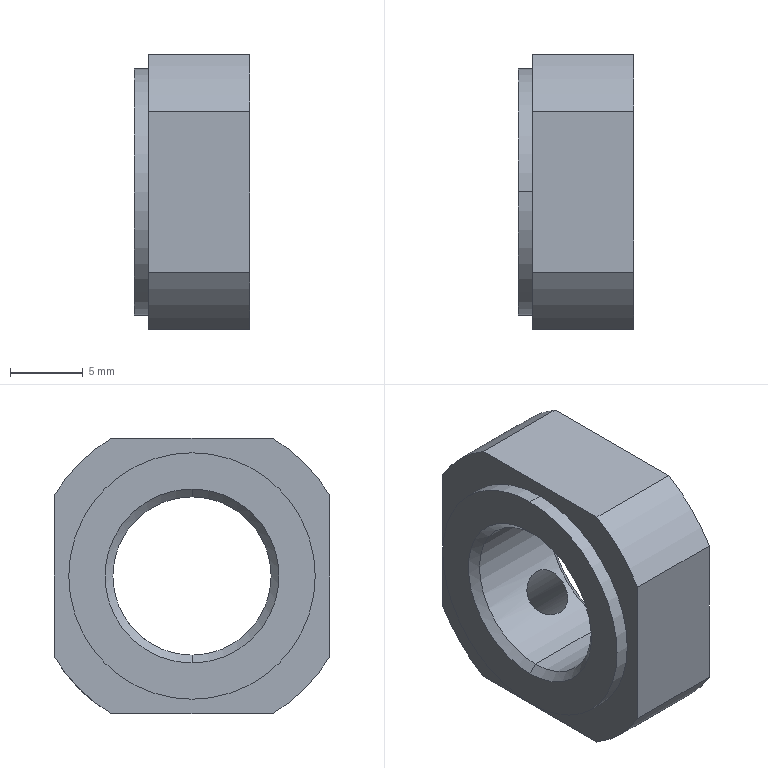Part | SolidWorks | features BaseBody 1 | 1 solid | 23 faces | box 8 x 19 x 19 mm | volume 1767 mm3 | cylinder 10 | plane 7 | cone 6 | commonest cylinder face diameters 22 x4 3.242 x2 10.917 x2 17 x2
STEP:
#1=CARTESIAN_POINT('',(0.,5.545,-9.5));
#2=VERTEX_POINT('',#1);
#3=CARTESIAN_POINT('',(0.,9.5,-5.545));
#4=VERTEX_POINT('',#3);
#5=CARTESIAN_POINT('',(0.,0.,0.));
#6=DIRECTION('',(1.,0.,0.));
#7=DIRECTION('',(0.,0.,-1.));
#8=AXIS2_PLACEMENT_3D('',#5,#6,#7);
#9=CIRCLE('',#8,11.);
#10=EDGE_CURVE('',#2,#4,#9,.T.);
#11=ORIENTED_EDGE('',*,*,#10,.T.);
#12=CARTESIAN_POINT('',(7.,9.5,-5.545));
#13=VERTEX_POINT('',#12);
#14=CARTESIAN_POINT('',(7.,9.5,-5.545));
#15=DIRECTION('',(-1.,0.,0.));
#16=VECTOR('',#15,1000.);
#17=LINE('',#14,#16);
#18=EDGE_CURVE('',#13,#4,#17,.T.);
#19=ORIENTED_EDGE('',*,*,#18,.F.);
#20=CARTESIAN_POINT('',(7.,5.545,-9.5));
#21=VERTEX_POINT('',#20);
#22=CARTESIAN_POINT('',(7.,0.,0.));
#23=DIRECTION('',(1.,0.,0.));
#24=DIRECTION('',(0.,0.,-1.));
#25=AXIS2_PLACEMENT_3D('',#22,#23,#24);
#26=CIRCLE('',#25,11.);
#27=EDGE_CURVE('',#21,#13,#26,.T.);
#28=ORIENTED_EDGE('',*,*,#27,.F.);
#29=CARTESIAN_POINT('',(7.,5.545,-9.5));
#30=DIRECTION('',(-1.,0.,0.));
#31=VECTOR('',#30,1000.);
#32=LINE('',#29,#31);
#33=EDGE_CURVE('',#21,#2,#32,.T.);
#34=ORIENTED_EDGE('',*,*,#33,.T.);
#35=EDGE_LOOP('',(#11,#19,#28,#34));
#36=FACE_OUTER_BOUND('',#35,.T.);
#37=CARTESIAN_POINT('',(4.5,6.364,-8.972));
#38=VERTEX_POINT('',#37);
#39=CARTESIAN_POINT('',(2.966,6.897,-8.569));
#40=VERTEX_POINT('',#39);
#41=CARTESIAN_POINT('',(4.5,6.364,-8.972));
#42=CARTESIAN_POINT('',(4.212,6.364,-8.972));
#43=CARTESIAN_POINT('',(3.926,6.412,-8.939));
#44=CARTESIAN_POINT('',(3.398,6.596,-8.804));
#45=CARTESIAN_POINT('',(3.158,6.732,-8.702));
#46=CARTESIAN_POINT('',(2.966,6.897,-8.569));
#47=B_SPLINE_CURVE_WITH_KNOTS('',3,(#41,#42,#43,#44,#45,#46),.UNSPECIFIED.,.F.,.F.,(4,2,4),(0.8576,0.9288,1.),.UNSPECIFIED.);
#48=EDGE_CURVE('',#38,#40,#47,.T.);
#49=ORIENTED_EDGE('',*,*,#48,.F.);
#50=CARTESIAN_POINT('',(4.5,8.972,-6.364));
#51=VERTEX_POINT('',#50);
#52=CARTESIAN_POINT('',(4.5,8.972,-6.364));
#53=CARTESIAN_POINT('',(4.751,8.972,-6.364));
#54=CARTESIAN_POINT('',(5.004,8.946,-6.401));
#55=CARTESIAN_POINT('',(5.476,8.843,-6.543));
#56=CARTESIAN_POINT('',(5.697,8.765,-6.649));
#57=CARTESIAN_POINT('',(6.073,8.558,-6.913));
#58=CARTESIAN_POINT('',(6.228,8.428,-7.072));
#59=CARTESIAN_POINT('',(6.443,8.127,-7.417));
#60=CARTESIAN_POINT('',(6.5,7.956,-7.601));
#61=CARTESIAN_POINT('',(6.5,7.598,-7.958));
#62=CARTESIAN_POINT('',(6.442,7.414,-8.129));
#63=CARTESIAN_POINT('',(6.228,7.071,-8.429));
#64=CARTESIAN_POINT('',(6.072,6.913,-8.558));
#65=CARTESIAN_POINT('',(5.696,6.649,-8.765));
#66=CARTESIAN_POINT('',(5.476,6.544,-8.843));
#67=CARTESIAN_POINT('',(5.004,6.401,-8.946));
#68=CARTESIAN_POINT('',(4.753,6.364,-8.972));
#69=CARTESIAN_POINT('',(4.5,6.364,-8.972));
#70=B_SPLINE_CURVE_WITH_KNOTS('',3,(#52,#53,#54,#55,#56,#57,#58,#59,#60,#61,#62,#63,#64,#65,#66,#67,#68,#69),.UNSPECIFIED.,.F.,.F.,(4,2,2,2,2,2,2,2,4),(0.3577,0.4202,0.4827,0.5452,0.6076,0.6701,0.7326,0.7951,0.8576),.UNSPECIFIED.);
#71=EDGE_CURVE('',#51,#38,#70,.T.);
#72=ORIENTED_EDGE('',*,*,#71,.F.);
#73=CARTESIAN_POINT('',(2.966,6.897,-8.569));
#74=CARTESIAN_POINT('',(2.846,7.001,-8.485));
#75=CARTESIAN_POINT('',(2.744,7.118,-8.388));
#76=CARTESIAN_POINT('',(2.59,7.363,-8.174));
#77=CARTESIAN_POINT('',(2.538,7.493,-8.055));
#78=CARTESIAN_POINT('',(2.491,7.751,-7.808));
#79=CARTESIAN_POINT('',(2.497,7.879,-7.678));
#80=CARTESIAN_POINT('',(2.564,8.122,-7.42));
#81=CARTESIAN_POINT('',(2.626,8.237,-7.293));
#82=CARTESIAN_POINT('',(2.885,8.547,-6.932));
#83=CARTESIAN_POINT('',(3.151,8.707,-6.725));
#84=CARTESIAN_POINT('',(3.78,8.919,-6.44));
#85=CARTESIAN_POINT('',(4.14,8.972,-6.364));
#86=CARTESIAN_POINT('',(4.5,8.972,-6.364));
#87=B_SPLINE_CURVE_WITH_KNOTS('',3,(#73,#74,#75,#76,#77,#78,#79,#80,#81,#82,#83,#84,#85,#86),.UNSPECIFIED.,.F.,.F.,(4,2,2,2,2,2,4),(0.,0.04471,0.08942,0.1341,0.1788,0.2683,0.3577),.UNSPECIFIED.);
#88=EDGE_CURVE('',#40,#51,#87,.T.);
#89=ORIENTED_EDGE('',*,*,#88,.F.);
#90=EDGE_LOOP('',(#49,#72,#89));
#91=FACE_BOUND('',#90,.T.);
#92=CARTESIAN_POINT('',(7.,0.,0.));
#93=DIRECTION('',(-1.,0.,0.));
#94=DIRECTION('',(0.,-0.7071,0.7071));
#95=AXIS2_PLACEMENT_3D('',#92,#93,#94);
#96=CYLINDRICAL_SURFACE('',#95,11.);
#97=ADVANCED_FACE('',(#36,#91),#96,.T.);
#98=CARTESIAN_POINT('',(4.5,6.364,-8.656));
#99=VERTEX_POINT('',#98);
#100=CARTESIAN_POINT('',(4.5,6.364,-8.656));
#101=DIRECTION('',(0.,0.,-1.));
#102=VECTOR('',#101,1000.);
#103=LINE('',#100,#102);
#104=EDGE_CURVE('',#99,#38,#103,.T.);
#105=ORIENTED_EDGE('',*,*,#104,.T.);
#106=ORIENTED_EDGE('',*,*,#48,.T.);
#107=ORIENTED_EDGE('',*,*,#88,.T.);
#108=CARTESIAN_POINT('',(4.5,8.656,-6.364));
#109=VERTEX_POINT('',#108);
#110=CARTESIAN_POINT('',(4.5,8.656,-6.364));
#111=DIRECTION('',(0.,1.,0.));
#112=VECTOR('',#111,1000.);
#113=LINE('',#110,#112);
#114=EDGE_CURVE('',#109,#51,#113,.T.);
#115=ORIENTED_EDGE('',*,*,#114,.F.);
#116=CARTESIAN_POINT('',(4.5,7.51,-7.51));
#117=DIRECTION('',(0.,-0.7071,0.7071));
#118=DIRECTION('',(0.,-0.7071,-0.7071));
#119=AXIS2_PLACEMENT_3D('',#116,#117,#118);
#120=CIRCLE('',#119,1.621);
#121=EDGE_CURVE('',#109,#99,#120,.T.);
#122=ORIENTED_EDGE('',*,*,#121,.T.);
#123=EDGE_LOOP('',(#105,#106,#107,#115,#122));
#124=FACE_OUTER_BOUND('',#123,.T.);
#125=CARTESIAN_POINT('',(4.5,7.778,-7.778));
#126=DIRECTION('',(0.,0.7071,-0.7071));
#127=DIRECTION('',(1.,0.,0.));
#128=AXIS2_PLACEMENT_3D('',#125,#126,#127);
#129=CONICAL_SURFACE('',#128,2.,0.7854);
#130=ADVANCED_FACE('',(#124),#129,.F.);
#131=CARTESIAN_POINT('',(4.5,4.832,-2.539));
#132=VERTEX_POINT('',#131);
#133=CARTESIAN_POINT('',(4.5,8.656,-6.364));
#134=DIRECTION('',(0.,-0.7071,0.7071));
#135=VECTOR('',#134,1000.);
#136=LINE('',#133,#135);
#137=EDGE_CURVE('',#109,#132,#136,.T.);
#138=ORIENTED_EDGE('',*,*,#137,.T.);
#139=CARTESIAN_POINT('',(4.5,2.539,-4.832));
#140=VERTEX_POINT('',#139);
#141=CARTESIAN_POINT('',(4.5,2.539,-4.832));
#142=CARTESIAN_POINT('',(4.288,2.539,-4.832));
#143=CARTESIAN_POINT('',(4.074,2.579,-4.811));
#144=CARTESIAN_POINT('',(3.682,2.728,-4.729));
#145=CARTESIAN_POINT('',(3.504,2.835,-4.667));
#146=CARTESIAN_POINT('',(3.205,3.091,-4.501));
#147=CARTESIAN_POINT('',(3.085,3.24,-4.398));
#148=CARTESIAN_POINT('',(2.922,3.549,-4.152));
#149=CARTESIAN_POINT('',(2.879,3.709,-4.011));
#150=CARTESIAN_POINT('',(2.879,4.011,-3.708));
#151=CARTESIAN_POINT('',(2.922,4.153,-3.548));
#152=CARTESIAN_POINT('',(3.085,4.397,-3.24));
#153=CARTESIAN_POINT('',(3.205,4.501,-3.091));
#154=CARTESIAN_POINT('',(3.503,4.667,-2.835));
#155=CARTESIAN_POINT('',(3.681,4.729,-2.728));
#156=CARTESIAN_POINT('',(4.074,4.811,-2.58));
#157=CARTESIAN_POINT('',(4.286,4.832,-2.54));
#158=CARTESIAN_POINT('',(4.5,4.832,-2.539));
#159=B_SPLINE_CURVE_WITH_KNOTS('',3,(#141,#142,#143,#144,#145,#146,#147,#148,#149,#150,#151,#152,#153,#154,#155,#156,#157,#158),.UNSPECIFIED.,.F.,.F.,(4,2,2,2,2,2,2,2,4),(0.,0.0625,0.125,0.1875,0.25,0.3125,0.375,0.4375,0.5),.UNSPECIFIED.);
#160=EDGE_CURVE('',#140,#132,#159,.T.);
#161=ORIENTED_EDGE('',*,*,#160,.F.);
#162=CARTESIAN_POINT('',(4.5,6.364,-8.656));
#163=DIRECTION('',(0.,-0.7071,0.7071));
#164=VECTOR('',#163,1000.);
#165=LINE('',#162,#164);
#166=EDGE_CURVE('',#99,#140,#165,.T.);
#167=ORIENTED_EDGE('',*,*,#166,.F.);
#168=ORIENTED_EDGE('',*,*,#121,.F.);
#169=EDGE_LOOP('',(#138,#161,#167,#168));
#170=FACE_OUTER_BOUND('',#169,.T.);
#171=CARTESIAN_POINT('',(4.5,0.,0.));
#172=DIRECTION('',(0.,-0.7071,0.7071));
#173=DIRECTION('',(1.,0.,0.));
#174=AXIS2_PLACEMENT_3D('',#171,#172,#173);
#175=CYLINDRICAL_SURFACE('',#174,1.621);
#176=ADVANCED_FACE('',(#170),#175,.F.);
#177=ORIENTED_EDGE('',*,*,#137,.F.);
#178=CARTESIAN_POINT('',(4.5,7.51,-7.51));
#179=DIRECTION('',(0.,-0.7071,0.7071));
#180=DIRECTION('',(0.,-0.7071,-0.7071));
#181=AXIS2_PLACEMENT_3D('',#178,#179,#180);
#182=CIRCLE('',#181,1.621);
#183=EDGE_CURVE('',#99,#109,#182,.T.);
#184=ORIENTED_EDGE('',*,*,#183,.F.);
#185=ORIENTED_EDGE('',*,*,#166,.T.);
#186=CARTESIAN_POINT('',(4.5,4.832,-2.539));
#187=CARTESIAN_POINT('',(4.714,4.832,-2.54));
#188=CARTESIAN_POINT('',(4.926,4.811,-2.58));
#189=CARTESIAN_POINT('',(5.319,4.729,-2.728));
#190=CARTESIAN_POINT('',(5.497,4.667,-2.835));
#191=CARTESIAN_POINT('',(5.795,4.502,-3.091));
#192=CARTESIAN_POINT('',(5.916,4.397,-3.241));
#193=CARTESIAN_POINT('',(6.078,4.153,-3.548));
#194=CARTESIAN_POINT('',(6.121,4.011,-3.709));
#195=CARTESIAN_POINT('',(6.121,3.709,-4.011));
#196=CARTESIAN_POINT('',(6.078,3.549,-4.152));
#197=CARTESIAN_POINT('',(5.915,3.24,-4.398));
#198=CARTESIAN_POINT('',(5.795,3.091,-4.501));
#199=CARTESIAN_POINT('',(5.496,2.835,-4.667));
#200=CARTESIAN_POINT('',(5.318,2.728,-4.729));
#201=CARTESIAN_POINT('',(4.926,2.579,-4.811));
#202=CARTESIAN_POINT('',(4.712,2.539,-4.832));
#203=CARTESIAN_POINT('',(4.5,2.539,-4.832));
#204=B_SPLINE_CURVE_WITH_KNOTS('',3,(#186,#187,#188,#189,#190,#191,#192,#193,#194,#195,#196,#197,#198,#199,#200,#201,#202,#203),.UNSPECIFIED.,.F.,.F.,(4,2,2,2,2,2,2,2,4),(0.5,0.5625,0.625,0.6875,0.75,0.8125,0.875,0.9375,1.),.UNSPECIFIED.);
#205=EDGE_CURVE('',#132,#140,#204,.T.);
#206=ORIENTED_EDGE('',*,*,#205,.F.);
#207=EDGE_LOOP('',(#177,#184,#185,#206));
#208=FACE_OUTER_BOUND('',#207,.T.);
#209=CARTESIAN_POINT('',(4.5,0.,0.));
#210=DIRECTION('',(0.,-0.7071,0.7071));
#211=DIRECTION('',(-1.,0.,0.));
#212=AXIS2_PLACEMENT_3D('',#209,#210,#211);
#213=CYLINDRICAL_SURFACE('',#212,1.621);
#214=ADVANCED_FACE('',(#208),#213,.F.);
#215=CARTESIAN_POINT('',(-0.4585,0.,5.458));
#216=VERTEX_POINT('',#215);
#217=CARTESIAN_POINT('',(6.459,0.,5.458));
#218=VERTEX_POINT('',#217);
#219=CARTESIAN_POINT('',(-0.4585,0.,5.458));
#220=DIRECTION('',(1.,0.,0.));
#221=VECTOR('',#220,1000.);
#222=LINE('',#219,#221);
#223=EDGE_CURVE('',#216,#218,#222,.T.);
#224=ORIENTED_EDGE('',*,*,#223,.F.);
#225=CARTESIAN_POINT('',(-0.4585,0.,-5.458));
#226=VERTEX_POINT('',#225);
#227=CARTESIAN_POINT('',(-0.4585,0.,0.));
#228=DIRECTION('',(1.,0.,0.));
#229=DIRECTION('',(0.,0.,-1.));
#230=AXIS2_PLACEMENT_3D('',#227,#228,#229);
#231=CIRCLE('',#230,5.458);
#232=EDGE_CURVE('',#226,#216,#231,.T.);
#233=ORIENTED_EDGE('',*,*,#232,.F.);
#234=CARTESIAN_POINT('',(6.458,0.,-5.458));
#235=VERTEX_POINT('',#234);
#236=CARTESIAN_POINT('',(-0.4585,0.,-5.458));
#237=DIRECTION('',(1.,0.,0.));
#238=VECTOR('',#237,1000.);
#239=LINE('',#236,#238);
#240=EDGE_CURVE('',#226,#235,#239,.T.);
#241=ORIENTED_EDGE('',*,*,#240,.T.);
#242=CARTESIAN_POINT('',(6.458,0.,0.));
#243=DIRECTION('',(1.,0.,0.));
#244=DIRECTION('',(0.,0.,-1.));
#245=AXIS2_PLACEMENT_3D('',#242,#243,#244);
#246=CIRCLE('',#245,5.458);
#247=EDGE_CURVE('',#235,#218,#246,.T.);
#248=ORIENTED_EDGE('',*,*,#247,.T.);
#249=EDGE_LOOP('',(#224,#233,#241,#248));
#250=FACE_OUTER_BOUND('',#249,.T.);
#251=ORIENTED_EDGE('',*,*,#160,.T.);
#252=ORIENTED_EDGE('',*,*,#205,.T.);
#253=EDGE_LOOP('',(#251,#252));
#254=FACE_BOUND('',#253,.T.);
#255=CARTESIAN_POINT('',(7.,0.,0.));
#256=DIRECTION('',(1.,0.,0.));
#257=DIRECTION('',(0.,-1.,0.));
#258=AXIS2_PLACEMENT_3D('',#255,#256,#257);
#259=CYLINDRICAL_SURFACE('',#258,5.458);
#260=ADVANCED_FACE('',(#250,#254),#259,.F.);
#261=CARTESIAN_POINT('',(7.,0.,6.));
#262=VERTEX_POINT('',#261);
#263=CARTESIAN_POINT('',(6.458,0.,5.458));
#264=DIRECTION('',(0.7071,0.,0.7071));
#265=VECTOR('',#264,1000.);
#266=LINE('',#263,#265);
#267=EDGE_CURVE('',#218,#262,#266,.T.);
#268=ORIENTED_EDGE('',*,*,#267,.F.);
#269=ORIENTED_EDGE('',*,*,#247,.F.);
#270=CARTESIAN_POINT('',(7.,0.,-6.));
#271=VERTEX_POINT('',#270);
#272=CARTESIAN_POINT('',(6.458,0.,-5.458));
#273=DIRECTION('',(0.7071,0.,-0.7071));
#274=VECTOR('',#273,1000.);
#275=LINE('',#272,#274);
#276=EDGE_CURVE('',#235,#271,#275,.T.);
#277=ORIENTED_EDGE('',*,*,#276,.T.);
#278=CARTESIAN_POINT('',(7.,0.,0.));
#279=DIRECTION('',(1.,0.,0.));
#280=DIRECTION('',(0.,0.,-1.));
#281=AXIS2_PLACEMENT_3D('',#278,#279,#280);
#282=CIRCLE('',#281,6.);
#283=EDGE_CURVE('',#271,#262,#282,.T.);
#284=ORIENTED_EDGE('',*,*,#283,.T.);
#285=EDGE_LOOP('',(#268,#269,#277,#284));
#286=FACE_OUTER_BOUND('',#285,.T.);
#287=CARTESIAN_POINT('',(6.458,0.,0.));
#288=DIRECTION('',(1.,0.,0.));
#289=DIRECTION('',(0.,-1.,0.));
#290=AXIS2_PLACEMENT_3D('',#287,#288,#289);
#291=CONICAL_SURFACE('',#290,5.458,0.7854);
#292=ADVANCED_FACE('',(#286),#291,.F.);
#293=CARTESIAN_POINT('',(7.,0.,0.));
#294=DIRECTION('',(1.,0.,0.));
#295=DIRECTION('',(0.,0.,-1.));
#296=AXIS2_PLACEMENT_3D('',#293,#294,#295);
#297=CIRCLE('',#296,6.);
#298=EDGE_CURVE('',#262,#271,#297,.T.);
#299=ORIENTED_EDGE('',*,*,#298,.F.);
#300=ORIENTED_EDGE('',*,*,#283,.F.);
#301=EDGE_LOOP('',(#299,#300));
#302=FACE_BOUND('',#301,.T.);
#303=CARTESIAN_POINT('',(7.,9.5,5.545));
#304=VERTEX_POINT('',#303);
#305=CARTESIAN_POINT('',(7.,5.545,9.5));
#306=VERTEX_POINT('',#305);
#307=CARTESIAN_POINT('',(7.,0.,0.));
#308=DIRECTION('',(1.,0.,0.));
#309=DIRECTION('',(0.,0.,-1.));
#310=AXIS2_PLACEMENT_3D('',#307,#308,#309);
#311=CIRCLE('',#310,11.);
#312=EDGE_CURVE('',#304,#306,#311,.T.);
#313=ORIENTED_EDGE('',*,*,#312,.T.);
#314=CARTESIAN_POINT('',(7.,-5.545,9.5));
#315=VERTEX_POINT('',#314);
#316=CARTESIAN_POINT('',(7.,5.545,9.5));
#317=DIRECTION('',(0.,-1.,0.));
#318=VECTOR('',#317,1000.);
#319=LINE('',#316,#318);
#320=EDGE_CURVE('',#306,#315,#319,.T.);
#321=ORIENTED_EDGE('',*,*,#320,.T.);
#322=CARTESIAN_POINT('',(7.,-9.5,5.545));
#323=VERTEX_POINT('',#322);
#324=CARTESIAN_POINT('',(7.,0.,0.));
#325=DIRECTION('',(1.,0.,0.));
#326=DIRECTION('',(0.,0.,-1.));
#327=AXIS2_PLACEMENT_3D('',#324,#325,#326);
#328=CIRCLE('',#327,11.);
#329=EDGE_CURVE('',#315,#323,#328,.T.);
#330=ORIENTED_EDGE('',*,*,#329,.T.);
#331=CARTESIAN_POINT('',(7.,-9.5,-5.545));
#332=VERTEX_POINT('',#331);
#333=CARTESIAN_POINT('',(7.,-9.5,5.545));
#334=DIRECTION('',(0.,0.,-1.));
#335=VECTOR('',#334,1000.);
#336=LINE('',#333,#335);
#337=EDGE_CURVE('',#323,#332,#336,.T.);
#338=ORIENTED_EDGE('',*,*,#337,.T.);
#339=CARTESIAN_POINT('',(7.,-5.545,-9.5));
#340=VERTEX_POINT('',#339);
#341=CARTESIAN_POINT('',(7.,0.,0.));
#342=DIRECTION('',(1.,0.,0.));
#343=DIRECTION('',(0.,0.,-1.));
#344=AXIS2_PLACEMENT_3D('',#341,#342,#343);
#345=CIRCLE('',#344,11.);
#346=EDGE_CURVE('',#332,#340,#345,.T.);
#347=ORIENTED_EDGE('',*,*,#346,.T.);
#348=CARTESIAN_POINT('',(7.,-5.545,-9.5));
#349=DIRECTION('',(0.,1.,0.));
#350=VECTOR('',#349,1000.);
#351=LINE('',#348,#350);
#352=EDGE_CURVE('',#340,#21,#351,.T.);
#353=ORIENTED_EDGE('',*,*,#352,.T.);
#354=ORIENTED_EDGE('',*,*,#27,.T.);
#355=CARTESIAN_POINT('',(7.,9.5,-5.545));
#356=DIRECTION('',(0.,0.,1.));
#357=VECTOR('',#356,1000.);
#358=LINE('',#355,#357);
#359=EDGE_CURVE('',#13,#304,#358,.T.);
#360=ORIENTED_EDGE('',*,*,#359,.T.);
#361=EDGE_LOOP('',(#313,#321,#330,#338,#347,#353,#354,#360));
#362=FACE_OUTER_BOUND('',#361,.T.);
#363=CARTESIAN_POINT('',(7.,0.,0.));
#364=DIRECTION('',(1.,0.,0.));
#365=DIRECTION('',(0.,0.,-1.));
#366=AXIS2_PLACEMENT_3D('',#363,#364,#365);
#367=PLANE('',#366);
#368=ADVANCED_FACE('',(#302,#362),#367,.T.);
#369=CARTESIAN_POINT('',(0.,9.5,5.545));
#370=VERTEX_POINT('',#369);
#371=CARTESIAN_POINT('',(0.,9.5,-5.545));
#372=DIRECTION('',(0.,0.,1.));
#373=VECTOR('',#372,1000.);
#374=LINE('',#371,#373);
#375=EDGE_CURVE('',#4,#370,#374,.T.);
#376=ORIENTED_EDGE('',*,*,#375,.T.);
#377=CARTESIAN_POINT('',(7.,9.5,5.545));
#378=DIRECTION('',(-1.,0.,0.));
#379=VECTOR('',#378,1000.);
#380=LINE('',#377,#379);
#381=EDGE_CURVE('',#304,#370,#380,.T.);
#382=ORIENTED_EDGE('',*,*,#381,.F.);
#383=ORIENTED_EDGE('',*,*,#359,.F.);
#384=ORIENTED_EDGE('',*,*,#18,.T.);
#385=EDGE_LOOP('',(#376,#382,#383,#384));
#386=FACE_OUTER_BOUND('',#385,.T.);
#387=CARTESIAN_POINT('',(7.,9.5,-5.545));
#388=DIRECTION('',(0.,-1.,0.));
#389=DIRECTION('',(0.,0.,-1.));
#390=AXIS2_PLACEMENT_3D('',#387,#388,#389);
#391=PLANE('',#390);
#392=ADVANCED_FACE('',(#386),#391,.F.);
#393=CARTESIAN_POINT('',(0.,5.545,9.5));
#394=VERTEX_POINT('',#393);
#395=CARTESIAN_POINT('',(0.,0.,0.));
#396=DIRECTION('',(1.,0.,0.));
#397=DIRECTION('',(0.,0.,-1.));
#398=AXIS2_PLACEMENT_3D('',#395,#396,#397);
#399=CIRCLE('',#398,11.);
#400=EDGE_CURVE('',#370,#394,#399,.T.);
#401=ORIENTED_EDGE('',*,*,#400,.T.);
#402=CARTESIAN_POINT('',(7.,5.545,9.5));
#403=DIRECTION('',(-1.,0.,0.));
#404=VECTOR('',#403,1000.);
#405=LINE('',#402,#404);
#406=EDGE_CURVE('',#306,#394,#405,.T.);
#407=ORIENTED_EDGE('',*,*,#406,.F.);
#408=ORIENTED_EDGE('',*,*,#312,.F.);
#409=ORIENTED_EDGE('',*,*,#381,.T.);
#410=EDGE_LOOP('',(#401,#407,#408,#409));
#411=FACE_OUTER_BOUND('',#410,.T.);
#412=CARTESIAN_POINT('',(7.,0.,0.));
#413=DIRECTION('',(-1.,0.,0.));
#414=DIRECTION('',(0.,-0.7071,-0.7071));
#415=AXIS2_PLACEMENT_3D('',#412,#413,#414);
#416=CYLINDRICAL_SURFACE('',#415,11.);
#417=ADVANCED_FACE('',(#411),#416,.T.);
#418=CARTESIAN_POINT('',(0.,-5.545,9.5));
#419=VERTEX_POINT('',#418);
#420=CARTESIAN_POINT('',(0.,5.545,9.5));
#421=DIRECTION('',(0.,-1.,0.));
#422=VECTOR('',#421,1000.);
#423=LINE('',#420,#422);
#424=EDGE_CURVE('',#394,#419,#423,.T.);
#425=ORIENTED_EDGE('',*,*,#424,.T.);
#426=CARTESIAN_POINT('',(7.,-5.545,9.5));
#427=DIRECTION('',(-1.,0.,0.));
#428=VECTOR('',#427,1000.);
#429=LINE('',#426,#428);
#430=EDGE_CURVE('',#315,#419,#429,.T.);
#431=ORIENTED_EDGE('',*,*,#430,.F.);
#432=ORIENTED_EDGE('',*,*,#320,.F.);
#433=ORIENTED_EDGE('',*,*,#406,.T.);
#434=EDGE_LOOP('',(#425,#431,#432,#433));
#435=FACE_OUTER_BOUND('',#434,.T.);
#436=CARTESIAN_POINT('',(7.,5.545,9.5));
#437=DIRECTION('',(0.,0.,-1.));
#438=DIRECTION('',(-1.,0.,0.));
#439=AXIS2_PLACEMENT_3D('',#436,#437,#438);
#440=PLANE('',#439);
#441=ADVANCED_FACE('',(#435),#440,.F.);
#442=CARTESIAN_POINT('',(0.,-9.5,5.545));
#443=VERTEX_POINT('',#442);
#444=CARTESIAN_POINT('',(0.,0.,0.));
#445=DIRECTION('',(1.,0.,0.));
#446=DIRECTION('',(0.,0.,-1.));
#447=AXIS2_PLACEMENT_3D('',#444,#445,#446);
#448=CIRCLE('',#447,11.);
#449=EDGE_CURVE('',#419,#443,#448,.T.);
#450=ORIENTED_EDGE('',*,*,#449,.T.);
#451=CARTESIAN_POINT('',(7.,-9.5,5.545));
#452=DIRECTION('',(-1.,0.,0.));
#453=VECTOR('',#452,1000.);
#454=LINE('',#451,#453);
#455=EDGE_CURVE('',#323,#443,#454,.T.);
#456=ORIENTED_EDGE('',*,*,#455,.F.);
#457=ORIENTED_EDGE('',*,*,#329,.F.);
#458=ORIENTED_EDGE('',*,*,#430,.T.);
#459=EDGE_LOOP('',(#450,#456,#457,#458));
#460=FACE_OUTER_BOUND('',#459,.T.);
#461=CARTESIAN_POINT('',(7.,0.,0.));
#462=DIRECTION('',(-1.,0.,0.));
#463=DIRECTION('',(0.,0.7071,-0.7071));
#464=AXIS2_PLACEMENT_3D('',#461,#462,#463);
#465=CYLINDRICAL_SURFACE('',#464,11.);
#466=ADVANCED_FACE('',(#460),#465,.T.);
#467=CARTESIAN_POINT('',(0.,-9.5,-5.545));
#468=VERTEX_POINT('',#467);
#469=CARTESIAN_POINT('',(0.,-9.5,5.545));
#470=DIRECTION('',(0.,0.,-1.));
#471=VECTOR('',#470,1000.);
#472=LINE('',#469,#471);
#473=EDGE_CURVE('',#443,#468,#472,.T.);
#474=ORIENTED_EDGE('',*,*,#473,.T.);
#475=CARTESIAN_POINT('',(7.,-9.5,-5.545));
#476=DIRECTION('',(-1.,0.,0.));
#477=VECTOR('',#476,1000.);
#478=LINE('',#475,#477);
#479=EDGE_CURVE('',#332,#468,#478,.T.);
#480=ORIENTED_EDGE('',*,*,#479,.F.);
#481=ORIENTED_EDGE('',*,*,#337,.F.);
#482=ORIENTED_EDGE('',*,*,#455,.T.);
#483=EDGE_LOOP('',(#474,#480,#481,#482));
#484=FACE_OUTER_BOUND('',#483,.T.);
#485=CARTESIAN_POINT('',(7.,-9.5,5.545));
#486=DIRECTION('',(0.,1.,0.));
#487=DIRECTION('',(0.,0.,1.));
#488=AXIS2_PLACEMENT_3D('',#485,#486,#487);
#489=PLANE('',#488);
#490=ADVANCED_FACE('',(#484),#489,.F.);
#491=CARTESIAN_POINT('',(0.,-5.545,-9.5));
#492=VERTEX_POINT('',#491);
#493=CARTESIAN_POINT('',(0.,0.,0.));
#494=DIRECTION('',(1.,0.,0.));
#495=DIRECTION('',(0.,0.,-1.));
#496=AXIS2_PLACEMENT_3D('',#493,#494,#495);
#497=CIRCLE('',#496,11.);
#498=EDGE_CURVE('',#468,#492,#497,.T.);
#499=ORIENTED_EDGE('',*,*,#498,.T.);
#500=CARTESIAN_POINT('',(7.,-5.545,-9.5));
#501=DIRECTION('',(-1.,0.,0.));
#502=VECTOR('',#501,1000.);
#503=LINE('',#500,#502);
#504=EDGE_CURVE('',#340,#492,#503,.T.);
#505=ORIENTED_EDGE('',*,*,#504,.F.);
#506=ORIENTED_EDGE('',*,*,#346,.F.);
#507=ORIENTED_EDGE('',*,*,#479,.T.);
#508=EDGE_LOOP('',(#499,#505,#506,#507));
#509=FACE_OUTER_BOUND('',#508,.T.);
#510=CARTESIAN_POINT('',(7.,0.,0.));
#511=DIRECTION('',(-1.,0.,0.));
#512=DIRECTION('',(0.,0.7071,0.7071));
#513=AXIS2_PLACEMENT_3D('',#510,#511,#512);
#514=CYLINDRICAL_SURFACE('',#513,11.);
#515=ADVANCED_FACE('',(#509),#514,.T.);
#516=CARTESIAN_POINT('',(0.,-5.545,-9.5));
#517=DIRECTION('',(0.,1.,0.));
#518=VECTOR('',#517,1000.);
#519=LINE('',#516,#518);
#520=EDGE_CURVE('',#492,#2,#519,.T.);
#521=ORIENTED_EDGE('',*,*,#520,.T.);
#522=ORIENTED_EDGE('',*,*,#33,.F.);
#523=ORIENTED_EDGE('',*,*,#352,.F.);
#524=ORIENTED_EDGE('',*,*,#504,.T.);
#525=EDGE_LOOP('',(#521,#522,#523,#524));
#526=FACE_OUTER_BOUND('',#525,.T.);
#527=CARTESIAN_POINT('',(7.,-5.545,-9.5));
#528=DIRECTION('',(0.,0.,1.));
#529=DIRECTION('',(1.,0.,0.));
#530=AXIS2_PLACEMENT_3D('',#527,#528,#529);
#531=PLANE('',#530);
#532=ADVANCED_FACE('',(#526),#531,.F.);
#533=CARTESIAN_POINT('',(0.,0.,8.5));
#534=VERTEX_POINT('',#533);
#535=CARTESIAN_POINT('',(0.,0.,-8.5));
#536=VERTEX_POINT('',#535);
#537=CARTESIAN_POINT('',(0.,0.,0.));
#538=DIRECTION('',(-1.,0.,0.));
#539=DIRECTION('',(0.,0.,-1.));
#540=AXIS2_PLACEMENT_3D('',#537,#538,#539);
#541=CIRCLE('',#540,8.5);
#542=EDGE_CURVE('',#534,#536,#541,.T.);
#543=ORIENTED_EDGE('',*,*,#542,.F.);
#544=CARTESIAN_POINT('',(0.,0.,0.));
#545=DIRECTION('',(-1.,0.,0.));
#546=DIRECTION('',(0.,0.,-1.));
#547=AXIS2_PLACEMENT_3D('',#544,#545,#546);
#548=CIRCLE('',#547,8.5);
#549=EDGE_CURVE('',#536,#534,#548,.T.);
#550=ORIENTED_EDGE('',*,*,#549,.F.);
#551=EDGE_LOOP('',(#543,#550));
#552=FACE_BOUND('',#551,.T.);
#553=ORIENTED_EDGE('',*,*,#400,.F.);
#554=ORIENTED_EDGE('',*,*,#375,.F.);
#555=ORIENTED_EDGE('',*,*,#10,.F.);
#556=ORIENTED_EDGE('',*,*,#520,.F.);
#557=ORIENTED_EDGE('',*,*,#498,.F.);
#558=ORIENTED_EDGE('',*,*,#473,.F.);
#559=ORIENTED_EDGE('',*,*,#449,.F.);
#560=ORIENTED_EDGE('',*,*,#424,.F.);
#561=EDGE_LOOP('',(#553,#554,#555,#556,#557,#558,#559,#560));
#562=FACE_OUTER_BOUND('',#561,.T.);
#563=CARTESIAN_POINT('',(0.,0.,0.));
#564=DIRECTION('',(1.,0.,0.));
#565=DIRECTION('',(0.,0.,-1.));
#566=AXIS2_PLACEMENT_3D('',#563,#564,#565);
#567=PLANE('',#566);
#568=ADVANCED_FACE('',(#552,#562),#567,.F.);
#569=CARTESIAN_POINT('',(-1.,0.,8.5));
#570=VERTEX_POINT('',#569);
#571=CARTESIAN_POINT('',(-1.,0.,8.5));
#572=DIRECTION('',(1.,0.,0.));
#573=VECTOR('',#572,1000.);
#574=LINE('',#571,#573);
#575=EDGE_CURVE('',#570,#534,#574,.T.);
#576=ORIENTED_EDGE('',*,*,#575,.F.);
#577=CARTESIAN_POINT('',(-1.,0.,-8.5));
#578=VERTEX_POINT('',#577);
#579=CARTESIAN_POINT('',(-1.,0.,0.));
#580=DIRECTION('',(1.,0.,0.));
#581=DIRECTION('',(0.,0.,-1.));
#582=AXIS2_PLACEMENT_3D('',#579,#580,#581);
#583=CIRCLE('',#582,8.5);
#584=EDGE_CURVE('',#570,#578,#583,.T.);
#585=ORIENTED_EDGE('',*,*,#584,.T.);
#586=CARTESIAN_POINT('',(-1.,0.,-8.5));
#587=DIRECTION('',(1.,0.,0.));
#588=VECTOR('',#587,1000.);
#589=LINE('',#586,#588);
#590=EDGE_CURVE('',#578,#536,#589,.T.);
#591=ORIENTED_EDGE('',*,*,#590,.T.);
#592=ORIENTED_EDGE('',*,*,#549,.T.);
#593=EDGE_LOOP('',(#576,#585,#591,#592));
#594=FACE_OUTER_BOUND('',#593,.T.);
#595=CARTESIAN_POINT('',(0.,0.,0.));
#596=DIRECTION('',(1.,0.,0.));
#597=DIRECTION('',(0.,1.,0.));
#598=AXIS2_PLACEMENT_3D('',#595,#596,#597);
#599=CYLINDRICAL_SURFACE('',#598,8.5);
#600=ADVANCED_FACE('',(#594),#599,.T.);
#601=ORIENTED_EDGE('',*,*,#575,.T.);
#602=ORIENTED_EDGE('',*,*,#542,.T.);
#603=ORIENTED_EDGE('',*,*,#590,.F.);
#604=CARTESIAN_POINT('',(-1.,0.,0.));
#605=DIRECTION('',(1.,0.,0.));
#606=DIRECTION('',(0.,0.,-1.));
#607=AXIS2_PLACEMENT_3D('',#604,#605,#606);
#608=CIRCLE('',#607,8.5);
#609=EDGE_CURVE('',#578,#570,#608,.T.);
#610=ORIENTED_EDGE('',*,*,#609,.T.);
#611=EDGE_LOOP('',(#601,#602,#603,#610));
#612=FACE_OUTER_BOUND('',#611,.T.);
#613=CARTESIAN_POINT('',(0.,0.,0.));
#614=DIRECTION('',(1.,0.,0.));
#615=DIRECTION('',(0.,-1.,0.));
#616=AXIS2_PLACEMENT_3D('',#613,#614,#615);
#617=CYLINDRICAL_SURFACE('',#616,8.5);
#618=ADVANCED_FACE('',(#612),#617,.T.);
#619=ORIENTED_EDGE('',*,*,#584,.F.);
#620=ORIENTED_EDGE('',*,*,#609,.F.);
#621=EDGE_LOOP('',(#619,#620));
#622=FACE_OUTER_BOUND('',#621,.T.);
#623=CARTESIAN_POINT('',(-1.,0.,-6.));
#624=VERTEX_POINT('',#623);
#625=CARTESIAN_POINT('',(-1.,0.,6.));
#626=VERTEX_POINT('',#625);
#627=CARTESIAN_POINT('',(-1.,0.,0.));
#628=DIRECTION('',(1.,0.,0.));
#629=DIRECTION('',(0.,0.,-1.));
#630=AXIS2_PLACEMENT_3D('',#627,#628,#629);
#631=CIRCLE('',#630,6.);
#632=EDGE_CURVE('',#624,#626,#631,.T.);
#633=ORIENTED_EDGE('',*,*,#632,.T.);
#634=CARTESIAN_POINT('',(-1.,0.,0.));
#635=DIRECTION('',(1.,0.,0.));
#636=DIRECTION('',(0.,0.,-1.));
#637=AXIS2_PLACEMENT_3D('',#634,#635,#636);
#638=CIRCLE('',#637,6.);
#639=EDGE_CURVE('',#626,#624,#638,.T.);
#640=ORIENTED_EDGE('',*,*,#639,.T.);
#641=EDGE_LOOP('',(#633,#640));
#642=FACE_BOUND('',#641,.T.);
#643=CARTESIAN_POINT('',(-1.,0.,0.));
#644=DIRECTION('',(1.,0.,0.));
#645=DIRECTION('',(0.,0.,-1.));
#646=AXIS2_PLACEMENT_3D('',#643,#644,#645);
#647=PLANE('',#646);
#648=ADVANCED_FACE('',(#622,#642),#647,.F.);
#649=CARTESIAN_POINT('',(-0.4585,0.,-5.458));
#650=DIRECTION('',(-0.7071,0.,-0.7071));
#651=VECTOR('',#650,1000.);
#652=LINE('',#649,#651);
#653=EDGE_CURVE('',#226,#624,#652,.T.);
#654=ORIENTED_EDGE('',*,*,#653,.T.);
#655=ORIENTED_EDGE('',*,*,#639,.F.);
#656=CARTESIAN_POINT('',(-0.4585,0.,5.458));
#657=DIRECTION('',(-0.7071,0.,0.7071));
#658=VECTOR('',#657,1000.);
#659=LINE('',#656,#658);
#660=EDGE_CURVE('',#216,#626,#659,.T.);
#661=ORIENTED_EDGE('',*,*,#660,.F.);
#662=CARTESIAN_POINT('',(-0.4585,0.,0.));
#663=DIRECTION('',(1.,0.,0.));
#664=DIRECTION('',(0.,0.,-1.));
#665=AXIS2_PLACEMENT_3D('',#662,#663,#664);
#666=CIRCLE('',#665,5.458);
#667=EDGE_CURVE('',#216,#226,#666,.T.);
#668=ORIENTED_EDGE('',*,*,#667,.T.);
#669=EDGE_LOOP('',(#654,#655,#661,#668));
#670=FACE_OUTER_BOUND('',#669,.T.);
#671=CARTESIAN_POINT('',(-1.,0.,0.));
#672=DIRECTION('',(-1.,0.,0.));
#673=DIRECTION('',(0.,1.,0.));
#674=AXIS2_PLACEMENT_3D('',#671,#672,#673);
#675=CONICAL_SURFACE('',#674,6.,0.7854);
#676=ADVANCED_FACE('',(#670),#675,.F.);
#677=ORIENTED_EDGE('',*,*,#223,.T.);
#678=CARTESIAN_POINT('',(6.458,0.,0.));
#679=DIRECTION('',(1.,0.,0.));
#680=DIRECTION('',(0.,0.,-1.));
#681=AXIS2_PLACEMENT_3D('',#678,#679,#680);
#682=CIRCLE('',#681,5.458);
#683=EDGE_CURVE('',#218,#235,#682,.T.);
#684=ORIENTED_EDGE('',*,*,#683,.T.);
#685=ORIENTED_EDGE('',*,*,#240,.F.);
#686=ORIENTED_EDGE('',*,*,#667,.F.);
#687=EDGE_LOOP('',(#677,#684,#685,#686));
#688=FACE_OUTER_BOUND('',#687,.T.);
#689=CARTESIAN_POINT('',(7.,0.,0.));
#690=DIRECTION('',(1.,0.,0.));
#691=DIRECTION('',(0.,1.,0.));
#692=AXIS2_PLACEMENT_3D('',#689,#690,#691);
#693=CYLINDRICAL_SURFACE('',#692,5.458);
#694=ADVANCED_FACE('',(#688),#693,.F.);
#695=ORIENTED_EDGE('',*,*,#267,.T.);
#696=ORIENTED_EDGE('',*,*,#298,.T.);
#697=ORIENTED_EDGE('',*,*,#276,.F.);
#698=ORIENTED_EDGE('',*,*,#683,.F.);
#699=EDGE_LOOP('',(#695,#696,#697,#698));
#700=FACE_OUTER_BOUND('',#699,.T.);
#701=CARTESIAN_POINT('',(6.458,0.,0.));
#702=DIRECTION('',(1.,0.,0.));
#703=DIRECTION('',(0.,1.,0.));
#704=AXIS2_PLACEMENT_3D('',#701,#702,#703);
#705=CONICAL_SURFACE('',#704,5.458,0.7854);
#706=ADVANCED_FACE('',(#700),#705,.F.);
#707=ORIENTED_EDGE('',*,*,#653,.F.);
#708=ORIENTED_EDGE('',*,*,#232,.T.);
#709=ORIENTED_EDGE('',*,*,#660,.T.);
#710=ORIENTED_EDGE('',*,*,#632,.F.);
#711=EDGE_LOOP('',(#707,#708,#709,#710));
#712=FACE_OUTER_BOUND('',#711,.T.);
#713=CARTESIAN_POINT('',(-1.,0.,0.));
#714=DIRECTION('',(-1.,0.,0.));
#715=DIRECTION('',(0.,-1.,0.));
#716=AXIS2_PLACEMENT_3D('',#713,#714,#715);
#717=CONICAL_SURFACE('',#716,6.,0.7854);
#718=ADVANCED_FACE('',(#712),#717,.F.);
#719=ORIENTED_EDGE('',*,*,#104,.F.);
#720=ORIENTED_EDGE('',*,*,#183,.T.);
#721=ORIENTED_EDGE('',*,*,#114,.T.);
#722=ORIENTED_EDGE('',*,*,#71,.T.);
#723=EDGE_LOOP('',(#719,#720,#721,#722));
#724=FACE_OUTER_BOUND('',#723,.T.);
#725=CARTESIAN_POINT('',(4.5,7.778,-7.778));
#726=DIRECTION('',(0.,0.7071,-0.7071));
#727=DIRECTION('',(-1.,0.,0.));
#728=AXIS2_PLACEMENT_3D('',#725,#726,#727);
#729=CONICAL_SURFACE('',#728,2.,0.7854);
#730=ADVANCED_FACE('',(#724),#729,.F.);
#731=CLOSED_SHELL('',(#97,#130,#176,#214,#260,#292,#368,#392,#417,#441,#466,#490,#515,#532,#568,#600,#618,#648,#676,#694,#706,#718,#730));
#732=MANIFOLD_SOLID_BREP('',#731);
#733=CARTESIAN_POINT('',(0.,0.,0.));
#734=DIRECTION('',(0.,0.,1.));
#735=DIRECTION('',(1.,0.,0.));
#736=AXIS2_PLACEMENT_3D('',#733,#734,#735);
#737=(LENGTH_UNIT()NAMED_UNIT(*)SI_UNIT(.MILLI.,.METRE.));
#738=UNCERTAINTY_MEASURE_WITH_UNIT(LENGTH_MEASURE(0.00001),#737,'','');
#739=(NAMED_UNIT(*)PLANE_ANGLE_UNIT()SI_UNIT($,.RADIAN.));
#740=(NAMED_UNIT(*)SI_UNIT($,.STERADIAN.)SOLID_ANGLE_UNIT());
#741=(GEOMETRIC_REPRESENTATION_CONTEXT(3)GLOBAL_UNCERTAINTY_ASSIGNED_CONTEXT((#738))GLOBAL_UNIT_ASSIGNED_CONTEXT((#737,#739,#740))REPRESENTATION_CONTEXT('',''));
#742=ADVANCED_BREP_SHAPE_REPRESENTATION('',(#732,#736),#741);